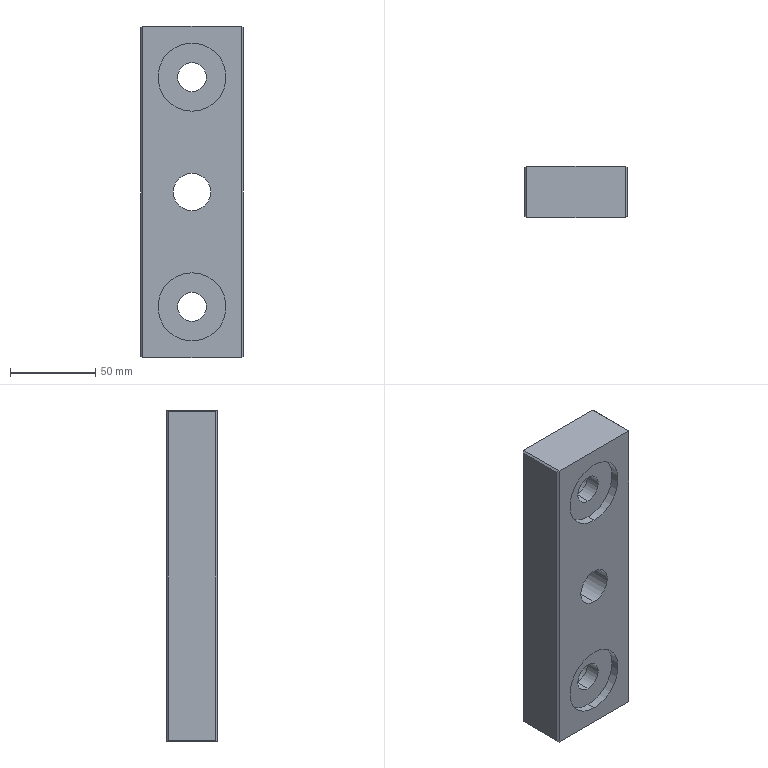Part | SolidWorks | features BaseBody 1 | 1 solid | 38 faces | box 60 x 30 x 195 mm | volume 305388 mm3 | plane 18 | cylinder 14 | cone 6 | commonest cylinder face diameters 17 x4 26 x4 40 x4 22 x2
STEP:
#1=CARTESIAN_POINT('',(0.,14.,-80.5));
#2=VERTEX_POINT('',#1);
#3=CARTESIAN_POINT('',(0.,14.,-54.5));
#4=VERTEX_POINT('',#3);
#5=CARTESIAN_POINT('',(0.,14.,-67.5));
#6=DIRECTION('',(0.,1.,0.));
#7=DIRECTION('',(0.,0.,-1.));
#8=AXIS2_PLACEMENT_3D('',#5,#6,#7);
#9=CIRCLE('',#8,13.);
#10=EDGE_CURVE('',#2,#4,#9,.T.);
#11=ORIENTED_EDGE('',*,*,#10,.F.);
#12=CARTESIAN_POINT('',(0.,15.,-81.5));
#13=VERTEX_POINT('',#12);
#14=CARTESIAN_POINT('',(0.,14.,-80.5));
#15=DIRECTION('',(0.,0.7071,-0.7071));
#16=VECTOR('',#15,1000.);
#17=LINE('',#14,#16);
#18=EDGE_CURVE('',#2,#13,#17,.T.);
#19=ORIENTED_EDGE('',*,*,#18,.T.);
#20=CARTESIAN_POINT('',(0.,15.,-53.5));
#21=VERTEX_POINT('',#20);
#22=CARTESIAN_POINT('',(0.,15.,-67.5));
#23=DIRECTION('',(0.,-1.,0.));
#24=DIRECTION('',(0.,0.,-1.));
#25=AXIS2_PLACEMENT_3D('',#22,#23,#24);
#26=CIRCLE('',#25,14.);
#27=EDGE_CURVE('',#21,#13,#26,.T.);
#28=ORIENTED_EDGE('',*,*,#27,.F.);
#29=CARTESIAN_POINT('',(0.,14.,-54.5));
#30=DIRECTION('',(0.,0.7071,0.7071));
#31=VECTOR('',#30,1000.);
#32=LINE('',#29,#31);
#33=EDGE_CURVE('',#4,#21,#32,.T.);
#34=ORIENTED_EDGE('',*,*,#33,.F.);
#35=EDGE_LOOP('',(#11,#19,#28,#34));
#36=FACE_OUTER_BOUND('',#35,.T.);
#37=CARTESIAN_POINT('',(0.,14.,-67.5));
#38=DIRECTION('',(0.,1.,0.));
#39=DIRECTION('',(0.,0.,1.));
#40=AXIS2_PLACEMENT_3D('',#37,#38,#39);
#41=CONICAL_SURFACE('',#40,13.,0.7854);
#42=ADVANCED_FACE('',(#36),#41,.F.);
#43=CARTESIAN_POINT('',(0.,14.,-11.));
#44=VERTEX_POINT('',#43);
#45=CARTESIAN_POINT('',(0.,14.,11.));
#46=VERTEX_POINT('',#45);
#47=CARTESIAN_POINT('',(0.,14.,0.));
#48=DIRECTION('',(0.,1.,0.));
#49=DIRECTION('',(0.,0.,-1.));
#50=AXIS2_PLACEMENT_3D('',#47,#48,#49);
#51=CIRCLE('',#50,11.);
#52=EDGE_CURVE('',#44,#46,#51,.T.);
#53=ORIENTED_EDGE('',*,*,#52,.F.);
#54=CARTESIAN_POINT('',(0.,15.,-12.));
#55=VERTEX_POINT('',#54);
#56=CARTESIAN_POINT('',(0.,14.,-11.));
#57=DIRECTION('',(0.,0.7071,-0.7071));
#58=VECTOR('',#57,1000.);
#59=LINE('',#56,#58);
#60=EDGE_CURVE('',#44,#55,#59,.T.);
#61=ORIENTED_EDGE('',*,*,#60,.T.);
#62=CARTESIAN_POINT('',(0.,15.,12.));
#63=VERTEX_POINT('',#62);
#64=CARTESIAN_POINT('',(0.,15.,0.));
#65=DIRECTION('',(0.,-1.,0.));
#66=DIRECTION('',(0.,0.,-1.));
#67=AXIS2_PLACEMENT_3D('',#64,#65,#66);
#68=CIRCLE('',#67,12.);
#69=EDGE_CURVE('',#63,#55,#68,.T.);
#70=ORIENTED_EDGE('',*,*,#69,.F.);
#71=CARTESIAN_POINT('',(0.,14.,11.));
#72=DIRECTION('',(0.,0.7071,0.7071));
#73=VECTOR('',#72,1000.);
#74=LINE('',#71,#73);
#75=EDGE_CURVE('',#46,#63,#74,.T.);
#76=ORIENTED_EDGE('',*,*,#75,.F.);
#77=EDGE_LOOP('',(#53,#61,#70,#76));
#78=FACE_OUTER_BOUND('',#77,.T.);
#79=CARTESIAN_POINT('',(0.,14.,0.));
#80=DIRECTION('',(0.,1.,0.));
#81=DIRECTION('',(0.,0.,1.));
#82=AXIS2_PLACEMENT_3D('',#79,#80,#81);
#83=CONICAL_SURFACE('',#82,11.,0.7854);
#84=ADVANCED_FACE('',(#78),#83,.F.);
#85=CARTESIAN_POINT('',(0.,14.,54.5));
#86=VERTEX_POINT('',#85);
#87=CARTESIAN_POINT('',(0.,14.,80.5));
#88=VERTEX_POINT('',#87);
#89=CARTESIAN_POINT('',(0.,14.,67.5));
#90=DIRECTION('',(0.,1.,0.));
#91=DIRECTION('',(0.,0.,-1.));
#92=AXIS2_PLACEMENT_3D('',#89,#90,#91);
#93=CIRCLE('',#92,13.);
#94=EDGE_CURVE('',#86,#88,#93,.T.);
#95=ORIENTED_EDGE('',*,*,#94,.F.);
#96=CARTESIAN_POINT('',(0.,15.,53.5));
#97=VERTEX_POINT('',#96);
#98=CARTESIAN_POINT('',(0.,14.,54.5));
#99=DIRECTION('',(0.,0.7071,-0.7071));
#100=VECTOR('',#99,1000.);
#101=LINE('',#98,#100);
#102=EDGE_CURVE('',#86,#97,#101,.T.);
#103=ORIENTED_EDGE('',*,*,#102,.T.);
#104=CARTESIAN_POINT('',(0.,15.,81.5));
#105=VERTEX_POINT('',#104);
#106=CARTESIAN_POINT('',(0.,15.,67.5));
#107=DIRECTION('',(0.,-1.,0.));
#108=DIRECTION('',(0.,0.,-1.));
#109=AXIS2_PLACEMENT_3D('',#106,#107,#108);
#110=CIRCLE('',#109,14.);
#111=EDGE_CURVE('',#105,#97,#110,.T.);
#112=ORIENTED_EDGE('',*,*,#111,.F.);
#113=CARTESIAN_POINT('',(0.,14.,80.5));
#114=DIRECTION('',(0.,0.7071,0.7071));
#115=VECTOR('',#114,1000.);
#116=LINE('',#113,#115);
#117=EDGE_CURVE('',#88,#105,#116,.T.);
#118=ORIENTED_EDGE('',*,*,#117,.F.);
#119=EDGE_LOOP('',(#95,#103,#112,#118));
#120=FACE_OUTER_BOUND('',#119,.T.);
#121=CARTESIAN_POINT('',(0.,14.,67.5));
#122=DIRECTION('',(0.,1.,0.));
#123=DIRECTION('',(0.,0.,1.));
#124=AXIS2_PLACEMENT_3D('',#121,#122,#123);
#125=CONICAL_SURFACE('',#124,13.,0.7854);
#126=ADVANCED_FACE('',(#120),#125,.F.);
#127=CARTESIAN_POINT('',(0.,-1.,-80.5));
#128=VERTEX_POINT('',#127);
#129=CARTESIAN_POINT('',(0.,-1.,-54.5));
#130=VERTEX_POINT('',#129);
#131=CARTESIAN_POINT('',(0.,-1.,-67.5));
#132=DIRECTION('',(0.,1.,0.));
#133=DIRECTION('',(0.,0.,1.));
#134=AXIS2_PLACEMENT_3D('',#131,#132,#133);
#135=CIRCLE('',#134,13.);
#136=EDGE_CURVE('',#128,#130,#135,.T.);
#137=ORIENTED_EDGE('',*,*,#136,.F.);
#138=CARTESIAN_POINT('',(0.,-1.,-80.5));
#139=DIRECTION('',(0.,1.,0.));
#140=VECTOR('',#139,1000.);
#141=LINE('',#138,#140);
#142=EDGE_CURVE('',#128,#2,#141,.T.);
#143=ORIENTED_EDGE('',*,*,#142,.T.);
#144=ORIENTED_EDGE('',*,*,#10,.T.);
#145=CARTESIAN_POINT('',(0.,-1.,-54.5));
#146=DIRECTION('',(0.,1.,0.));
#147=VECTOR('',#146,1000.);
#148=LINE('',#145,#147);
#149=EDGE_CURVE('',#130,#4,#148,.T.);
#150=ORIENTED_EDGE('',*,*,#149,.F.);
#151=EDGE_LOOP('',(#137,#143,#144,#150));
#152=FACE_OUTER_BOUND('',#151,.T.);
#153=CARTESIAN_POINT('',(0.,-1.,-67.5));
#154=DIRECTION('',(0.,1.,0.));
#155=DIRECTION('',(0.,0.,1.));
#156=AXIS2_PLACEMENT_3D('',#153,#154,#155);
#157=CYLINDRICAL_SURFACE('',#156,13.);
#158=ADVANCED_FACE('',(#152),#157,.F.);
#159=CARTESIAN_POINT('',(0.,-1.,54.5));
#160=VERTEX_POINT('',#159);
#161=CARTESIAN_POINT('',(0.,-1.,80.5));
#162=VERTEX_POINT('',#161);
#163=CARTESIAN_POINT('',(0.,-1.,67.5));
#164=DIRECTION('',(0.,1.,0.));
#165=DIRECTION('',(0.,0.,1.));
#166=AXIS2_PLACEMENT_3D('',#163,#164,#165);
#167=CIRCLE('',#166,13.);
#168=EDGE_CURVE('',#160,#162,#167,.T.);
#169=ORIENTED_EDGE('',*,*,#168,.F.);
#170=CARTESIAN_POINT('',(0.,-1.,54.5));
#171=DIRECTION('',(0.,1.,0.));
#172=VECTOR('',#171,1000.);
#173=LINE('',#170,#172);
#174=EDGE_CURVE('',#160,#86,#173,.T.);
#175=ORIENTED_EDGE('',*,*,#174,.T.);
#176=ORIENTED_EDGE('',*,*,#94,.T.);
#177=CARTESIAN_POINT('',(0.,-1.,80.5));
#178=DIRECTION('',(0.,1.,0.));
#179=VECTOR('',#178,1000.);
#180=LINE('',#177,#179);
#181=EDGE_CURVE('',#162,#88,#180,.T.);
#182=ORIENTED_EDGE('',*,*,#181,.F.);
#183=EDGE_LOOP('',(#169,#175,#176,#182));
#184=FACE_OUTER_BOUND('',#183,.T.);
#185=CARTESIAN_POINT('',(0.,-1.,67.5));
#186=DIRECTION('',(0.,1.,0.));
#187=DIRECTION('',(0.,0.,1.));
#188=AXIS2_PLACEMENT_3D('',#185,#186,#187);
#189=CYLINDRICAL_SURFACE('',#188,13.);
#190=ADVANCED_FACE('',(#184),#189,.F.);
#191=CARTESIAN_POINT('',(0.,-10.,87.5));
#192=VERTEX_POINT('',#191);
#193=CARTESIAN_POINT('',(0.,-10.,47.5));
#194=VERTEX_POINT('',#193);
#195=CARTESIAN_POINT('',(0.,-10.,67.5));
#196=DIRECTION('',(0.,-1.,0.));
#197=DIRECTION('',(0.,0.,-1.));
#198=AXIS2_PLACEMENT_3D('',#195,#196,#197);
#199=CIRCLE('',#198,20.);
#200=EDGE_CURVE('',#192,#194,#199,.T.);
#201=ORIENTED_EDGE('',*,*,#200,.F.);
#202=CARTESIAN_POINT('',(0.,-15.,87.5));
#203=VERTEX_POINT('',#202);
#204=CARTESIAN_POINT('',(0.,-10.,87.5));
#205=DIRECTION('',(0.,-1.,0.));
#206=VECTOR('',#205,1000.);
#207=LINE('',#204,#206);
#208=EDGE_CURVE('',#192,#203,#207,.T.);
#209=ORIENTED_EDGE('',*,*,#208,.T.);
#210=CARTESIAN_POINT('',(0.,-15.,47.5));
#211=VERTEX_POINT('',#210);
#212=CARTESIAN_POINT('',(0.,-15.,67.5));
#213=DIRECTION('',(0.,-1.,0.));
#214=DIRECTION('',(0.,0.,-1.));
#215=AXIS2_PLACEMENT_3D('',#212,#213,#214);
#216=CIRCLE('',#215,20.);
#217=EDGE_CURVE('',#203,#211,#216,.T.);
#218=ORIENTED_EDGE('',*,*,#217,.T.);
#219=CARTESIAN_POINT('',(0.,-10.,47.5));
#220=DIRECTION('',(0.,-1.,0.));
#221=VECTOR('',#220,1000.);
#222=LINE('',#219,#221);
#223=EDGE_CURVE('',#194,#211,#222,.T.);
#224=ORIENTED_EDGE('',*,*,#223,.F.);
#225=EDGE_LOOP('',(#201,#209,#218,#224));
#226=FACE_OUTER_BOUND('',#225,.T.);
#227=CARTESIAN_POINT('',(0.,-10.,67.5));
#228=DIRECTION('',(0.,-1.,0.));
#229=DIRECTION('',(0.,0.,-1.));
#230=AXIS2_PLACEMENT_3D('',#227,#228,#229);
#231=CYLINDRICAL_SURFACE('',#230,20.);
#232=ADVANCED_FACE('',(#226),#231,.F.);
#233=CARTESIAN_POINT('',(0.,-10.,-47.5));
#234=VERTEX_POINT('',#233);
#235=CARTESIAN_POINT('',(0.,-10.,-87.5));
#236=VERTEX_POINT('',#235);
#237=CARTESIAN_POINT('',(0.,-10.,-67.5));
#238=DIRECTION('',(0.,-1.,0.));
#239=DIRECTION('',(0.,0.,-1.));
#240=AXIS2_PLACEMENT_3D('',#237,#238,#239);
#241=CIRCLE('',#240,20.);
#242=EDGE_CURVE('',#234,#236,#241,.T.);
#243=ORIENTED_EDGE('',*,*,#242,.F.);
#244=CARTESIAN_POINT('',(0.,-15.,-47.5));
#245=VERTEX_POINT('',#244);
#246=CARTESIAN_POINT('',(0.,-10.,-47.5));
#247=DIRECTION('',(0.,-1.,0.));
#248=VECTOR('',#247,1000.);
#249=LINE('',#246,#248);
#250=EDGE_CURVE('',#234,#245,#249,.T.);
#251=ORIENTED_EDGE('',*,*,#250,.T.);
#252=CARTESIAN_POINT('',(0.,-15.,-87.5));
#253=VERTEX_POINT('',#252);
#254=CARTESIAN_POINT('',(0.,-15.,-67.5));
#255=DIRECTION('',(0.,-1.,0.));
#256=DIRECTION('',(0.,0.,-1.));
#257=AXIS2_PLACEMENT_3D('',#254,#255,#256);
#258=CIRCLE('',#257,20.);
#259=EDGE_CURVE('',#245,#253,#258,.T.);
#260=ORIENTED_EDGE('',*,*,#259,.T.);
#261=CARTESIAN_POINT('',(0.,-10.,-87.5));
#262=DIRECTION('',(0.,-1.,0.));
#263=VECTOR('',#262,1000.);
#264=LINE('',#261,#263);
#265=EDGE_CURVE('',#236,#253,#264,.T.);
#266=ORIENTED_EDGE('',*,*,#265,.F.);
#267=EDGE_LOOP('',(#243,#251,#260,#266));
#268=FACE_OUTER_BOUND('',#267,.T.);
#269=CARTESIAN_POINT('',(0.,-10.,-67.5));
#270=DIRECTION('',(0.,-1.,0.));
#271=DIRECTION('',(0.,0.,-1.));
#272=AXIS2_PLACEMENT_3D('',#269,#270,#271);
#273=CYLINDRICAL_SURFACE('',#272,20.);
#274=ADVANCED_FACE('',(#268),#273,.F.);
#275=ORIENTED_EDGE('',*,*,#52,.T.);
#276=CARTESIAN_POINT('',(0.,-15.,11.));
#277=VERTEX_POINT('',#276);
#278=CARTESIAN_POINT('',(0.,15.,11.));
#279=DIRECTION('',(0.,-1.,0.));
#280=VECTOR('',#279,1000.);
#281=LINE('',#278,#280);
#282=EDGE_CURVE('',#46,#277,#281,.T.);
#283=ORIENTED_EDGE('',*,*,#282,.T.);
#284=CARTESIAN_POINT('',(0.,-15.,-11.));
#285=VERTEX_POINT('',#284);
#286=CARTESIAN_POINT('',(0.,-15.,0.));
#287=DIRECTION('',(0.,1.,0.));
#288=DIRECTION('',(0.,0.,1.));
#289=AXIS2_PLACEMENT_3D('',#286,#287,#288);
#290=CIRCLE('',#289,11.);
#291=EDGE_CURVE('',#285,#277,#290,.T.);
#292=ORIENTED_EDGE('',*,*,#291,.F.);
#293=CARTESIAN_POINT('',(0.,15.,-11.));
#294=DIRECTION('',(0.,-1.,0.));
#295=VECTOR('',#294,1000.);
#296=LINE('',#293,#295);
#297=EDGE_CURVE('',#44,#285,#296,.T.);
#298=ORIENTED_EDGE('',*,*,#297,.F.);
#299=EDGE_LOOP('',(#275,#283,#292,#298));
#300=FACE_OUTER_BOUND('',#299,.T.);
#301=CARTESIAN_POINT('',(0.,15.,0.));
#302=DIRECTION('',(0.,-1.,0.));
#303=DIRECTION('',(0.,0.,-1.));
#304=AXIS2_PLACEMENT_3D('',#301,#302,#303);
#305=CYLINDRICAL_SURFACE('',#304,11.);
#306=ADVANCED_FACE('',(#300),#305,.F.);
#307=CARTESIAN_POINT('',(0.,-1.,-76.));
#308=VERTEX_POINT('',#307);
#309=CARTESIAN_POINT('',(0.,-1.,-59.));
#310=VERTEX_POINT('',#309);
#311=CARTESIAN_POINT('',(0.,-1.,-67.5));
#312=DIRECTION('',(0.,1.,0.));
#313=DIRECTION('',(0.,0.,1.));
#314=AXIS2_PLACEMENT_3D('',#311,#312,#313);
#315=CIRCLE('',#314,8.5);
#316=EDGE_CURVE('',#308,#310,#315,.T.);
#317=ORIENTED_EDGE('',*,*,#316,.T.);
#318=CARTESIAN_POINT('',(0.,-10.,-59.));
#319=VERTEX_POINT('',#318);
#320=CARTESIAN_POINT('',(0.,15.,-59.));
#321=DIRECTION('',(0.,-1.,0.));
#322=VECTOR('',#321,1000.);
#323=LINE('',#320,#322);
#324=EDGE_CURVE('',#310,#319,#323,.T.);
#325=ORIENTED_EDGE('',*,*,#324,.T.);
#326=CARTESIAN_POINT('',(0.,-10.,-76.));
#327=VERTEX_POINT('',#326);
#328=CARTESIAN_POINT('',(0.,-10.,-67.5));
#329=DIRECTION('',(0.,-1.,0.));
#330=DIRECTION('',(0.,0.,-1.));
#331=AXIS2_PLACEMENT_3D('',#328,#329,#330);
#332=CIRCLE('',#331,8.5);
#333=EDGE_CURVE('',#319,#327,#332,.T.);
#334=ORIENTED_EDGE('',*,*,#333,.T.);
#335=CARTESIAN_POINT('',(0.,15.,-76.));
#336=DIRECTION('',(0.,-1.,0.));
#337=VECTOR('',#336,1000.);
#338=LINE('',#335,#337);
#339=EDGE_CURVE('',#308,#327,#338,.T.);
#340=ORIENTED_EDGE('',*,*,#339,.F.);
#341=EDGE_LOOP('',(#317,#325,#334,#340));
#342=FACE_OUTER_BOUND('',#341,.T.);
#343=CARTESIAN_POINT('',(0.,15.,-67.5));
#344=DIRECTION('',(0.,-1.,0.));
#345=DIRECTION('',(0.,0.,-1.));
#346=AXIS2_PLACEMENT_3D('',#343,#344,#345);
#347=CYLINDRICAL_SURFACE('',#346,8.5);
#348=ADVANCED_FACE('',(#342),#347,.F.);
#349=CARTESIAN_POINT('',(0.,-1.,59.));
#350=VERTEX_POINT('',#349);
#351=CARTESIAN_POINT('',(0.,-1.,76.));
#352=VERTEX_POINT('',#351);
#353=CARTESIAN_POINT('',(0.,-1.,67.5));
#354=DIRECTION('',(0.,1.,0.));
#355=DIRECTION('',(0.,0.,1.));
#356=AXIS2_PLACEMENT_3D('',#353,#354,#355);
#357=CIRCLE('',#356,8.5);
#358=EDGE_CURVE('',#350,#352,#357,.T.);
#359=ORIENTED_EDGE('',*,*,#358,.T.);
#360=CARTESIAN_POINT('',(0.,-10.,76.));
#361=VERTEX_POINT('',#360);
#362=CARTESIAN_POINT('',(0.,15.,76.));
#363=DIRECTION('',(0.,-1.,0.));
#364=VECTOR('',#363,1000.);
#365=LINE('',#362,#364);
#366=EDGE_CURVE('',#352,#361,#365,.T.);
#367=ORIENTED_EDGE('',*,*,#366,.T.);
#368=CARTESIAN_POINT('',(0.,-10.,59.));
#369=VERTEX_POINT('',#368);
#370=CARTESIAN_POINT('',(0.,-10.,67.5));
#371=DIRECTION('',(0.,-1.,0.));
#372=DIRECTION('',(0.,0.,-1.));
#373=AXIS2_PLACEMENT_3D('',#370,#371,#372);
#374=CIRCLE('',#373,8.5);
#375=EDGE_CURVE('',#361,#369,#374,.T.);
#376=ORIENTED_EDGE('',*,*,#375,.T.);
#377=CARTESIAN_POINT('',(0.,15.,59.));
#378=DIRECTION('',(0.,-1.,0.));
#379=VECTOR('',#378,1000.);
#380=LINE('',#377,#379);
#381=EDGE_CURVE('',#350,#369,#380,.T.);
#382=ORIENTED_EDGE('',*,*,#381,.F.);
#383=EDGE_LOOP('',(#359,#367,#376,#382));
#384=FACE_OUTER_BOUND('',#383,.T.);
#385=CARTESIAN_POINT('',(0.,15.,67.5));
#386=DIRECTION('',(0.,-1.,0.));
#387=DIRECTION('',(0.,0.,-1.));
#388=AXIS2_PLACEMENT_3D('',#385,#386,#387);
#389=CYLINDRICAL_SURFACE('',#388,8.5);
#390=ADVANCED_FACE('',(#384),#389,.F.);
#391=ORIENTED_EDGE('',*,*,#366,.F.);
#392=CARTESIAN_POINT('',(0.,-1.,67.5));
#393=DIRECTION('',(0.,1.,0.));
#394=DIRECTION('',(0.,0.,1.));
#395=AXIS2_PLACEMENT_3D('',#392,#393,#394);
#396=CIRCLE('',#395,8.5);
#397=EDGE_CURVE('',#352,#350,#396,.T.);
#398=ORIENTED_EDGE('',*,*,#397,.T.);
#399=ORIENTED_EDGE('',*,*,#381,.T.);
#400=CARTESIAN_POINT('',(0.,-10.,67.5));
#401=DIRECTION('',(0.,-1.,0.));
#402=DIRECTION('',(0.,0.,-1.));
#403=AXIS2_PLACEMENT_3D('',#400,#401,#402);
#404=CIRCLE('',#403,8.5);
#405=EDGE_CURVE('',#369,#361,#404,.T.);
#406=ORIENTED_EDGE('',*,*,#405,.T.);
#407=EDGE_LOOP('',(#391,#398,#399,#406));
#408=FACE_OUTER_BOUND('',#407,.T.);
#409=CARTESIAN_POINT('',(0.,15.,67.5));
#410=DIRECTION('',(0.,-1.,0.));
#411=DIRECTION('',(0.,0.,-1.));
#412=AXIS2_PLACEMENT_3D('',#409,#410,#411);
#413=CYLINDRICAL_SURFACE('',#412,8.5);
#414=ADVANCED_FACE('',(#408),#413,.F.);
#415=ORIENTED_EDGE('',*,*,#324,.F.);
#416=CARTESIAN_POINT('',(0.,-1.,-67.5));
#417=DIRECTION('',(0.,1.,0.));
#418=DIRECTION('',(0.,0.,1.));
#419=AXIS2_PLACEMENT_3D('',#416,#417,#418);
#420=CIRCLE('',#419,8.5);
#421=EDGE_CURVE('',#310,#308,#420,.T.);
#422=ORIENTED_EDGE('',*,*,#421,.T.);
#423=ORIENTED_EDGE('',*,*,#339,.T.);
#424=CARTESIAN_POINT('',(0.,-10.,-67.5));
#425=DIRECTION('',(0.,-1.,0.));
#426=DIRECTION('',(0.,0.,-1.));
#427=AXIS2_PLACEMENT_3D('',#424,#425,#426);
#428=CIRCLE('',#427,8.5);
#429=EDGE_CURVE('',#327,#319,#428,.T.);
#430=ORIENTED_EDGE('',*,*,#429,.T.);
#431=EDGE_LOOP('',(#415,#422,#423,#430));
#432=FACE_OUTER_BOUND('',#431,.T.);
#433=CARTESIAN_POINT('',(0.,15.,-67.5));
#434=DIRECTION('',(0.,-1.,0.));
#435=DIRECTION('',(0.,0.,-1.));
#436=AXIS2_PLACEMENT_3D('',#433,#434,#435);
#437=CYLINDRICAL_SURFACE('',#436,8.5);
#438=ADVANCED_FACE('',(#432),#437,.F.);
#439=ORIENTED_EDGE('',*,*,#111,.T.);
#440=CARTESIAN_POINT('',(0.,15.,67.5));
#441=DIRECTION('',(0.,-1.,0.));
#442=DIRECTION('',(0.,0.,-1.));
#443=AXIS2_PLACEMENT_3D('',#440,#441,#442);
#444=CIRCLE('',#443,14.);
#445=EDGE_CURVE('',#97,#105,#444,.T.);
#446=ORIENTED_EDGE('',*,*,#445,.T.);
#447=EDGE_LOOP('',(#439,#446));
#448=FACE_BOUND('',#447,.T.);
#449=ORIENTED_EDGE('',*,*,#69,.T.);
#450=CARTESIAN_POINT('',(0.,15.,0.));
#451=DIRECTION('',(0.,-1.,0.));
#452=DIRECTION('',(0.,0.,-1.));
#453=AXIS2_PLACEMENT_3D('',#450,#451,#452);
#454=CIRCLE('',#453,12.);
#455=EDGE_CURVE('',#55,#63,#454,.T.);
#456=ORIENTED_EDGE('',*,*,#455,.T.);
#457=EDGE_LOOP('',(#449,#456));
#458=FACE_BOUND('',#457,.T.);
#459=ORIENTED_EDGE('',*,*,#27,.T.);
#460=CARTESIAN_POINT('',(0.,15.,-67.5));
#461=DIRECTION('',(0.,-1.,0.));
#462=DIRECTION('',(0.,0.,-1.));
#463=AXIS2_PLACEMENT_3D('',#460,#461,#462);
#464=CIRCLE('',#463,14.);
#465=EDGE_CURVE('',#13,#21,#464,.T.);
#466=ORIENTED_EDGE('',*,*,#465,.T.);
#467=EDGE_LOOP('',(#459,#466));
#468=FACE_BOUND('',#467,.T.);
#469=CARTESIAN_POINT('',(-29.,15.,97.5));
#470=VERTEX_POINT('',#469);
#471=CARTESIAN_POINT('',(29.,15.,97.5));
#472=VERTEX_POINT('',#471);
#473=CARTESIAN_POINT('',(29.,15.,97.5));
#474=DIRECTION('',(1.,0.,0.));
#475=VECTOR('',#474,1000.);
#476=LINE('',#473,#475);
#477=EDGE_CURVE('',#470,#472,#476,.T.);
#478=ORIENTED_EDGE('',*,*,#477,.T.);
#479=CARTESIAN_POINT('',(29.,15.,-97.5));
#480=VERTEX_POINT('',#479);
#481=CARTESIAN_POINT('',(29.,15.,0.));
#482=DIRECTION('',(0.,0.,-1.));
#483=VECTOR('',#482,1000.);
#484=LINE('',#481,#483);
#485=EDGE_CURVE('',#472,#480,#484,.T.);
#486=ORIENTED_EDGE('',*,*,#485,.T.);
#487=CARTESIAN_POINT('',(-29.,15.,-97.5));
#488=VERTEX_POINT('',#487);
#489=CARTESIAN_POINT('',(-29.,15.,-97.5));
#490=DIRECTION('',(-1.,0.,0.));
#491=VECTOR('',#490,1000.);
#492=LINE('',#489,#491);
#493=EDGE_CURVE('',#480,#488,#492,.T.);
#494=ORIENTED_EDGE('',*,*,#493,.T.);
#495=CARTESIAN_POINT('',(-29.,15.,0.));
#496=DIRECTION('',(0.,0.,1.));
#497=VECTOR('',#496,1000.);
#498=LINE('',#495,#497);
#499=EDGE_CURVE('',#488,#470,#498,.T.);
#500=ORIENTED_EDGE('',*,*,#499,.T.);
#501=EDGE_LOOP('',(#478,#486,#494,#500));
#502=FACE_OUTER_BOUND('',#501,.T.);
#503=CARTESIAN_POINT('',(0.,15.,0.));
#504=DIRECTION('',(0.,-1.,0.));
#505=DIRECTION('',(0.,0.,-1.));
#506=AXIS2_PLACEMENT_3D('',#503,#504,#505);
#507=PLANE('',#506);
#508=ADVANCED_FACE('',(#448,#458,#468,#502),#507,.F.);
#509=CARTESIAN_POINT('',(0.,-15.,-67.5));
#510=DIRECTION('',(0.,-1.,0.));
#511=DIRECTION('',(0.,0.,-1.));
#512=AXIS2_PLACEMENT_3D('',#509,#510,#511);
#513=CIRCLE('',#512,20.);
#514=EDGE_CURVE('',#253,#245,#513,.T.);
#515=ORIENTED_EDGE('',*,*,#514,.F.);
#516=ORIENTED_EDGE('',*,*,#259,.F.);
#517=EDGE_LOOP('',(#515,#516));
#518=FACE_BOUND('',#517,.T.);
#519=CARTESIAN_POINT('',(0.,-15.,67.5));
#520=DIRECTION('',(0.,-1.,0.));
#521=DIRECTION('',(0.,0.,-1.));
#522=AXIS2_PLACEMENT_3D('',#519,#520,#521);
#523=CIRCLE('',#522,20.);
#524=EDGE_CURVE('',#211,#203,#523,.T.);
#525=ORIENTED_EDGE('',*,*,#524,.F.);
#526=ORIENTED_EDGE('',*,*,#217,.F.);
#527=EDGE_LOOP('',(#525,#526));
#528=FACE_BOUND('',#527,.T.);
#529=CARTESIAN_POINT('',(-29.,-15.,97.5));
#530=VERTEX_POINT('',#529);
#531=CARTESIAN_POINT('',(29.,-15.,97.5));
#532=VERTEX_POINT('',#531);
#533=CARTESIAN_POINT('',(29.,-15.,97.5));
#534=DIRECTION('',(1.,0.,0.));
#535=VECTOR('',#534,1000.);
#536=LINE('',#533,#535);
#537=EDGE_CURVE('',#530,#532,#536,.T.);
#538=ORIENTED_EDGE('',*,*,#537,.F.);
#539=CARTESIAN_POINT('',(-29.,-15.,-97.5));
#540=VERTEX_POINT('',#539);
#541=CARTESIAN_POINT('',(-29.,-15.,-96.5));
#542=DIRECTION('',(0.,0.,-1.));
#543=VECTOR('',#542,1000.);
#544=LINE('',#541,#543);
#545=EDGE_CURVE('',#530,#540,#544,.T.);
#546=ORIENTED_EDGE('',*,*,#545,.T.);
#547=CARTESIAN_POINT('',(29.,-15.,-97.5));
#548=VERTEX_POINT('',#547);
#549=CARTESIAN_POINT('',(-29.,-15.,-97.5));
#550=DIRECTION('',(-1.,0.,0.));
#551=VECTOR('',#550,1000.);
#552=LINE('',#549,#551);
#553=EDGE_CURVE('',#548,#540,#552,.T.);
#554=ORIENTED_EDGE('',*,*,#553,.F.);
#555=CARTESIAN_POINT('',(29.,-15.,96.5));
#556=DIRECTION('',(0.,0.,1.));
#557=VECTOR('',#556,1000.);
#558=LINE('',#555,#557);
#559=EDGE_CURVE('',#548,#532,#558,.T.);
#560=ORIENTED_EDGE('',*,*,#559,.T.);
#561=EDGE_LOOP('',(#538,#546,#554,#560));
#562=FACE_OUTER_BOUND('',#561,.T.);
#563=ORIENTED_EDGE('',*,*,#291,.T.);
#564=CARTESIAN_POINT('',(0.,-15.,0.));
#565=DIRECTION('',(0.,1.,0.));
#566=DIRECTION('',(0.,0.,1.));
#567=AXIS2_PLACEMENT_3D('',#564,#565,#566);
#568=CIRCLE('',#567,11.);
#569=EDGE_CURVE('',#277,#285,#568,.T.);
#570=ORIENTED_EDGE('',*,*,#569,.T.);
#571=EDGE_LOOP('',(#563,#570));
#572=FACE_BOUND('',#571,.T.);
#573=CARTESIAN_POINT('',(0.,-15.,0.));
#574=DIRECTION('',(0.,-1.,0.));
#575=DIRECTION('',(0.,0.,-1.));
#576=AXIS2_PLACEMENT_3D('',#573,#574,#575);
#577=PLANE('',#576);
#578=ADVANCED_FACE('',(#518,#528,#562,#572),#577,.T.);
#579=CARTESIAN_POINT('',(-29.,15.,-97.5));
#580=DIRECTION('',(0.,-1.,0.));
#581=VECTOR('',#580,1000.);
#582=LINE('',#579,#581);
#583=EDGE_CURVE('',#488,#540,#582,.T.);
#584=ORIENTED_EDGE('',*,*,#583,.T.);
#585=CARTESIAN_POINT('',(-30.,-14.,-96.5));
#586=VERTEX_POINT('',#585);
#587=CARTESIAN_POINT('',(-94.333,50.333,-32.167));
#588=DIRECTION('',(-0.5774,0.5774,0.5774));
#589=VECTOR('',#588,1000.);
#590=LINE('',#587,#589);
#591=EDGE_CURVE('',#540,#586,#590,.T.);
#592=ORIENTED_EDGE('',*,*,#591,.T.);
#593=CARTESIAN_POINT('',(-30.,14.,-96.5));
#594=VERTEX_POINT('',#593);
#595=CARTESIAN_POINT('',(-30.,15.,-96.5));
#596=DIRECTION('',(0.,-1.,0.));
#597=VECTOR('',#596,1000.);
#598=LINE('',#595,#597);
#599=EDGE_CURVE('',#594,#586,#598,.T.);
#600=ORIENTED_EDGE('',*,*,#599,.F.);
#601=CARTESIAN_POINT('',(-61.5,-17.5,-65.));
#602=DIRECTION('',(0.5774,0.5774,-0.5774));
#603=VECTOR('',#602,1000.);
#604=LINE('',#601,#603);
#605=EDGE_CURVE('',#594,#488,#604,.T.);
#606=ORIENTED_EDGE('',*,*,#605,.T.);
#607=EDGE_LOOP('',(#584,#592,#600,#606));
#608=FACE_OUTER_BOUND('',#607,.T.);
#609=CARTESIAN_POINT('',(-30.,15.,-96.5));
#610=DIRECTION('',(0.7071,0.,0.7071));
#611=DIRECTION('',(0.7071,0.,-0.7071));
#612=AXIS2_PLACEMENT_3D('',#609,#610,#611);
#613=PLANE('',#612);
#614=ADVANCED_FACE('',(#608),#613,.F.);
#615=ORIENTED_EDGE('',*,*,#599,.T.);
#616=CARTESIAN_POINT('',(-30.,-14.,96.5));
#617=VERTEX_POINT('',#616);
#618=CARTESIAN_POINT('',(-30.,-14.,96.5));
#619=DIRECTION('',(0.,0.,1.));
#620=VECTOR('',#619,1000.);
#621=LINE('',#618,#620);
#622=EDGE_CURVE('',#586,#617,#621,.T.);
#623=ORIENTED_EDGE('',*,*,#622,.T.);
#624=CARTESIAN_POINT('',(-30.,14.,96.5));
#625=VERTEX_POINT('',#624);
#626=CARTESIAN_POINT('',(-30.,15.,96.5));
#627=DIRECTION('',(0.,-1.,0.));
#628=VECTOR('',#627,1000.);
#629=LINE('',#626,#628);
#630=EDGE_CURVE('',#625,#617,#629,.T.);
#631=ORIENTED_EDGE('',*,*,#630,.F.);
#632=CARTESIAN_POINT('',(-30.,14.,96.5));
#633=DIRECTION('',(0.,0.,-1.));
#634=VECTOR('',#633,1000.);
#635=LINE('',#632,#634);
#636=EDGE_CURVE('',#625,#594,#635,.T.);
#637=ORIENTED_EDGE('',*,*,#636,.T.);
#638=EDGE_LOOP('',(#615,#623,#631,#637));
#639=FACE_OUTER_BOUND('',#638,.T.);
#640=CARTESIAN_POINT('',(-30.,15.,96.5));
#641=DIRECTION('',(1.,0.,0.));
#642=DIRECTION('',(0.,0.,-1.));
#643=AXIS2_PLACEMENT_3D('',#640,#641,#642);
#644=PLANE('',#643);
#645=ADVANCED_FACE('',(#639),#644,.F.);
#646=ORIENTED_EDGE('',*,*,#630,.T.);
#647=CARTESIAN_POINT('',(-30.,-14.,96.5));
#648=DIRECTION('',(0.5774,-0.5774,0.5774));
#649=VECTOR('',#648,1000.);
#650=LINE('',#647,#649);
#651=EDGE_CURVE('',#617,#530,#650,.T.);
#652=ORIENTED_EDGE('',*,*,#651,.T.);
#653=CARTESIAN_POINT('',(-29.,15.,97.5));
#654=DIRECTION('',(0.,-1.,0.));
#655=VECTOR('',#654,1000.);
#656=LINE('',#653,#655);
#657=EDGE_CURVE('',#470,#530,#656,.T.);
#658=ORIENTED_EDGE('',*,*,#657,.F.);
#659=CARTESIAN_POINT('',(-61.5,-17.5,65.));
#660=DIRECTION('',(-0.5774,-0.5774,-0.5774));
#661=VECTOR('',#660,1000.);
#662=LINE('',#659,#661);
#663=EDGE_CURVE('',#470,#625,#662,.T.);
#664=ORIENTED_EDGE('',*,*,#663,.T.);
#665=EDGE_LOOP('',(#646,#652,#658,#664));
#666=FACE_OUTER_BOUND('',#665,.T.);
#667=CARTESIAN_POINT('',(-29.,15.,97.5));
#668=DIRECTION('',(0.7071,0.,-0.7071));
#669=DIRECTION('',(-0.7071,0.,-0.7071));
#670=AXIS2_PLACEMENT_3D('',#667,#668,#669);
#671=PLANE('',#670);
#672=ADVANCED_FACE('',(#666),#671,.F.);
#673=ORIENTED_EDGE('',*,*,#537,.T.);
#674=CARTESIAN_POINT('',(29.,15.,97.5));
#675=DIRECTION('',(0.,-1.,0.));
#676=VECTOR('',#675,1000.);
#677=LINE('',#674,#676);
#678=EDGE_CURVE('',#472,#532,#677,.T.);
#679=ORIENTED_EDGE('',*,*,#678,.F.);
#680=ORIENTED_EDGE('',*,*,#477,.F.);
#681=ORIENTED_EDGE('',*,*,#657,.T.);
#682=EDGE_LOOP('',(#673,#679,#680,#681));
#683=FACE_OUTER_BOUND('',#682,.T.);
#684=CARTESIAN_POINT('',(29.,15.,97.5));
#685=DIRECTION('',(0.,0.,-1.));
#686=DIRECTION('',(-1.,0.,0.));
#687=AXIS2_PLACEMENT_3D('',#684,#685,#686);
#688=PLANE('',#687);
#689=ADVANCED_FACE('',(#683),#688,.F.);
#690=ORIENTED_EDGE('',*,*,#678,.T.);
#691=CARTESIAN_POINT('',(30.,-14.,96.5));
#692=VERTEX_POINT('',#691);
#693=CARTESIAN_POINT('',(94.333,50.333,32.167));
#694=DIRECTION('',(0.5774,0.5774,-0.5774));
#695=VECTOR('',#694,1000.);
#696=LINE('',#693,#695);
#697=EDGE_CURVE('',#532,#692,#696,.T.);
#698=ORIENTED_EDGE('',*,*,#697,.T.);
#699=CARTESIAN_POINT('',(30.,14.,96.5));
#700=VERTEX_POINT('',#699);
#701=CARTESIAN_POINT('',(30.,15.,96.5));
#702=DIRECTION('',(0.,-1.,0.));
#703=VECTOR('',#702,1000.);
#704=LINE('',#701,#703);
#705=EDGE_CURVE('',#700,#692,#704,.T.);
#706=ORIENTED_EDGE('',*,*,#705,.F.);
#707=CARTESIAN_POINT('',(61.5,-17.5,65.));
#708=DIRECTION('',(-0.5774,0.5774,0.5774));
#709=VECTOR('',#708,1000.);
#710=LINE('',#707,#709);
#711=EDGE_CURVE('',#700,#472,#710,.T.);
#712=ORIENTED_EDGE('',*,*,#711,.T.);
#713=EDGE_LOOP('',(#690,#698,#706,#712));
#714=FACE_OUTER_BOUND('',#713,.T.);
#715=CARTESIAN_POINT('',(30.,15.,96.5));
#716=DIRECTION('',(-0.7071,0.,-0.7071));
#717=DIRECTION('',(-0.7071,0.,0.7071));
#718=AXIS2_PLACEMENT_3D('',#715,#716,#717);
#719=PLANE('',#718);
#720=ADVANCED_FACE('',(#714),#719,.F.);
#721=ORIENTED_EDGE('',*,*,#705,.T.);
#722=CARTESIAN_POINT('',(30.,-14.,-96.5));
#723=VERTEX_POINT('',#722);
#724=CARTESIAN_POINT('',(30.,-14.,-96.5));
#725=DIRECTION('',(0.,0.,-1.));
#726=VECTOR('',#725,1000.);
#727=LINE('',#724,#726);
#728=EDGE_CURVE('',#692,#723,#727,.T.);
#729=ORIENTED_EDGE('',*,*,#728,.T.);
#730=CARTESIAN_POINT('',(30.,14.,-96.5));
#731=VERTEX_POINT('',#730);
#732=CARTESIAN_POINT('',(30.,15.,-96.5));
#733=DIRECTION('',(0.,-1.,0.));
#734=VECTOR('',#733,1000.);
#735=LINE('',#732,#734);
#736=EDGE_CURVE('',#731,#723,#735,.T.);
#737=ORIENTED_EDGE('',*,*,#736,.F.);
#738=CARTESIAN_POINT('',(30.,14.,-96.5));
#739=DIRECTION('',(0.,0.,1.));
#740=VECTOR('',#739,1000.);
#741=LINE('',#738,#740);
#742=EDGE_CURVE('',#731,#700,#741,.T.);
#743=ORIENTED_EDGE('',*,*,#742,.T.);
#744=EDGE_LOOP('',(#721,#729,#737,#743));
#745=FACE_OUTER_BOUND('',#744,.T.);
#746=CARTESIAN_POINT('',(30.,15.,-96.5));
#747=DIRECTION('',(-1.,0.,0.));
#748=DIRECTION('',(0.,0.,1.));
#749=AXIS2_PLACEMENT_3D('',#746,#747,#748);
#750=PLANE('',#749);
#751=ADVANCED_FACE('',(#745),#750,.F.);
#752=ORIENTED_EDGE('',*,*,#736,.T.);
#753=CARTESIAN_POINT('',(30.,-14.,-96.5));
#754=DIRECTION('',(-0.5774,-0.5774,-0.5774));
#755=VECTOR('',#754,1000.);
#756=LINE('',#753,#755);
#757=EDGE_CURVE('',#723,#548,#756,.T.);
#758=ORIENTED_EDGE('',*,*,#757,.T.);
#759=CARTESIAN_POINT('',(29.,15.,-97.5));
#760=DIRECTION('',(0.,-1.,0.));
#761=VECTOR('',#760,1000.);
#762=LINE('',#759,#761);
#763=EDGE_CURVE('',#480,#548,#762,.T.);
#764=ORIENTED_EDGE('',*,*,#763,.F.);
#765=CARTESIAN_POINT('',(61.5,-17.5,-65.));
#766=DIRECTION('',(0.5774,-0.5774,0.5774));
#767=VECTOR('',#766,1000.);
#768=LINE('',#765,#767);
#769=EDGE_CURVE('',#480,#731,#768,.T.);
#770=ORIENTED_EDGE('',*,*,#769,.T.);
#771=EDGE_LOOP('',(#752,#758,#764,#770));
#772=FACE_OUTER_BOUND('',#771,.T.);
#773=CARTESIAN_POINT('',(29.,15.,-97.5));
#774=DIRECTION('',(-0.7071,0.,0.7071));
#775=DIRECTION('',(0.7071,0.,0.7071));
#776=AXIS2_PLACEMENT_3D('',#773,#774,#775);
#777=PLANE('',#776);
#778=ADVANCED_FACE('',(#772),#777,.F.);
#779=ORIENTED_EDGE('',*,*,#553,.T.);
#780=ORIENTED_EDGE('',*,*,#583,.F.);
#781=ORIENTED_EDGE('',*,*,#493,.F.);
#782=ORIENTED_EDGE('',*,*,#763,.T.);
#783=EDGE_LOOP('',(#779,#780,#781,#782));
#784=FACE_OUTER_BOUND('',#783,.T.);
#785=CARTESIAN_POINT('',(-29.,15.,-97.5));
#786=DIRECTION('',(0.,0.,1.));
#787=DIRECTION('',(1.,0.,0.));
#788=AXIS2_PLACEMENT_3D('',#785,#786,#787);
#789=PLANE('',#788);
#790=ADVANCED_FACE('',(#784),#789,.F.);
#791=ORIENTED_EDGE('',*,*,#282,.F.);
#792=CARTESIAN_POINT('',(0.,14.,0.));
#793=DIRECTION('',(0.,1.,0.));
#794=DIRECTION('',(0.,0.,-1.));
#795=AXIS2_PLACEMENT_3D('',#792,#793,#794);
#796=CIRCLE('',#795,11.);
#797=EDGE_CURVE('',#46,#44,#796,.T.);
#798=ORIENTED_EDGE('',*,*,#797,.T.);
#799=ORIENTED_EDGE('',*,*,#297,.T.);
#800=ORIENTED_EDGE('',*,*,#569,.F.);
#801=EDGE_LOOP('',(#791,#798,#799,#800));
#802=FACE_OUTER_BOUND('',#801,.T.);
#803=CARTESIAN_POINT('',(0.,15.,0.));
#804=DIRECTION('',(0.,-1.,0.));
#805=DIRECTION('',(0.,0.,-1.));
#806=AXIS2_PLACEMENT_3D('',#803,#804,#805);
#807=CYLINDRICAL_SURFACE('',#806,11.);
#808=ADVANCED_FACE('',(#802),#807,.F.);
#809=ORIENTED_EDGE('',*,*,#250,.F.);
#810=CARTESIAN_POINT('',(0.,-10.,-67.5));
#811=DIRECTION('',(0.,-1.,0.));
#812=DIRECTION('',(0.,0.,-1.));
#813=AXIS2_PLACEMENT_3D('',#810,#811,#812);
#814=CIRCLE('',#813,20.);
#815=EDGE_CURVE('',#236,#234,#814,.T.);
#816=ORIENTED_EDGE('',*,*,#815,.F.);
#817=ORIENTED_EDGE('',*,*,#265,.T.);
#818=ORIENTED_EDGE('',*,*,#514,.T.);
#819=EDGE_LOOP('',(#809,#816,#817,#818));
#820=FACE_OUTER_BOUND('',#819,.T.);
#821=CARTESIAN_POINT('',(0.,-10.,-67.5));
#822=DIRECTION('',(0.,-1.,0.));
#823=DIRECTION('',(0.,0.,-1.));
#824=AXIS2_PLACEMENT_3D('',#821,#822,#823);
#825=CYLINDRICAL_SURFACE('',#824,20.);
#826=ADVANCED_FACE('',(#820),#825,.F.);
#827=ORIENTED_EDGE('',*,*,#429,.F.);
#828=ORIENTED_EDGE('',*,*,#333,.F.);
#829=EDGE_LOOP('',(#827,#828));
#830=FACE_BOUND('',#829,.T.);
#831=ORIENTED_EDGE('',*,*,#815,.T.);
#832=ORIENTED_EDGE('',*,*,#242,.T.);
#833=EDGE_LOOP('',(#831,#832));
#834=FACE_OUTER_BOUND('',#833,.T.);
#835=CARTESIAN_POINT('',(0.,-10.,-67.5));
#836=DIRECTION('',(0.,-1.,0.));
#837=DIRECTION('',(0.,0.,-1.));
#838=AXIS2_PLACEMENT_3D('',#835,#836,#837);
#839=PLANE('',#838);
#840=ADVANCED_FACE('',(#830,#834),#839,.T.);
#841=ORIENTED_EDGE('',*,*,#208,.F.);
#842=CARTESIAN_POINT('',(0.,-10.,67.5));
#843=DIRECTION('',(0.,-1.,0.));
#844=DIRECTION('',(0.,0.,-1.));
#845=AXIS2_PLACEMENT_3D('',#842,#843,#844);
#846=CIRCLE('',#845,20.);
#847=EDGE_CURVE('',#194,#192,#846,.T.);
#848=ORIENTED_EDGE('',*,*,#847,.F.);
#849=ORIENTED_EDGE('',*,*,#223,.T.);
#850=ORIENTED_EDGE('',*,*,#524,.T.);
#851=EDGE_LOOP('',(#841,#848,#849,#850));
#852=FACE_OUTER_BOUND('',#851,.T.);
#853=CARTESIAN_POINT('',(0.,-10.,67.5));
#854=DIRECTION('',(0.,-1.,0.));
#855=DIRECTION('',(0.,0.,-1.));
#856=AXIS2_PLACEMENT_3D('',#853,#854,#855);
#857=CYLINDRICAL_SURFACE('',#856,20.);
#858=ADVANCED_FACE('',(#852),#857,.F.);
#859=ORIENTED_EDGE('',*,*,#405,.F.);
#860=ORIENTED_EDGE('',*,*,#375,.F.);
#861=EDGE_LOOP('',(#859,#860));
#862=FACE_BOUND('',#861,.T.);
#863=ORIENTED_EDGE('',*,*,#847,.T.);
#864=ORIENTED_EDGE('',*,*,#200,.T.);
#865=EDGE_LOOP('',(#863,#864));
#866=FACE_OUTER_BOUND('',#865,.T.);
#867=CARTESIAN_POINT('',(0.,-10.,67.5));
#868=DIRECTION('',(0.,-1.,0.));
#869=DIRECTION('',(0.,0.,-1.));
#870=AXIS2_PLACEMENT_3D('',#867,#868,#869);
#871=PLANE('',#870);
#872=ADVANCED_FACE('',(#862,#866),#871,.T.);
#873=ORIENTED_EDGE('',*,*,#174,.F.);
#874=CARTESIAN_POINT('',(0.,-1.,67.5));
#875=DIRECTION('',(0.,1.,0.));
#876=DIRECTION('',(0.,0.,1.));
#877=AXIS2_PLACEMENT_3D('',#874,#875,#876);
#878=CIRCLE('',#877,13.);
#879=EDGE_CURVE('',#162,#160,#878,.T.);
#880=ORIENTED_EDGE('',*,*,#879,.F.);
#881=ORIENTED_EDGE('',*,*,#181,.T.);
#882=CARTESIAN_POINT('',(0.,14.,67.5));
#883=DIRECTION('',(0.,1.,0.));
#884=DIRECTION('',(0.,0.,-1.));
#885=AXIS2_PLACEMENT_3D('',#882,#883,#884);
#886=CIRCLE('',#885,13.);
#887=EDGE_CURVE('',#88,#86,#886,.T.);
#888=ORIENTED_EDGE('',*,*,#887,.T.);
#889=EDGE_LOOP('',(#873,#880,#881,#888));
#890=FACE_OUTER_BOUND('',#889,.T.);
#891=CARTESIAN_POINT('',(0.,-1.,67.5));
#892=DIRECTION('',(0.,1.,0.));
#893=DIRECTION('',(0.,0.,1.));
#894=AXIS2_PLACEMENT_3D('',#891,#892,#893);
#895=CYLINDRICAL_SURFACE('',#894,13.);
#896=ADVANCED_FACE('',(#890),#895,.F.);
#897=ORIENTED_EDGE('',*,*,#358,.F.);
#898=ORIENTED_EDGE('',*,*,#397,.F.);
#899=EDGE_LOOP('',(#897,#898));
#900=FACE_BOUND('',#899,.T.);
#901=ORIENTED_EDGE('',*,*,#879,.T.);
#902=ORIENTED_EDGE('',*,*,#168,.T.);
#903=EDGE_LOOP('',(#901,#902));
#904=FACE_OUTER_BOUND('',#903,.T.);
#905=CARTESIAN_POINT('',(0.,-1.,67.5));
#906=DIRECTION('',(0.,1.,0.));
#907=DIRECTION('',(0.,0.,1.));
#908=AXIS2_PLACEMENT_3D('',#905,#906,#907);
#909=PLANE('',#908);
#910=ADVANCED_FACE('',(#900,#904),#909,.T.);
#911=ORIENTED_EDGE('',*,*,#142,.F.);
#912=CARTESIAN_POINT('',(0.,-1.,-67.5));
#913=DIRECTION('',(0.,1.,0.));
#914=DIRECTION('',(0.,0.,1.));
#915=AXIS2_PLACEMENT_3D('',#912,#913,#914);
#916=CIRCLE('',#915,13.);
#917=EDGE_CURVE('',#130,#128,#916,.T.);
#918=ORIENTED_EDGE('',*,*,#917,.F.);
#919=ORIENTED_EDGE('',*,*,#149,.T.);
#920=CARTESIAN_POINT('',(0.,14.,-67.5));
#921=DIRECTION('',(0.,1.,0.));
#922=DIRECTION('',(0.,0.,-1.));
#923=AXIS2_PLACEMENT_3D('',#920,#921,#922);
#924=CIRCLE('',#923,13.);
#925=EDGE_CURVE('',#4,#2,#924,.T.);
#926=ORIENTED_EDGE('',*,*,#925,.T.);
#927=EDGE_LOOP('',(#911,#918,#919,#926));
#928=FACE_OUTER_BOUND('',#927,.T.);
#929=CARTESIAN_POINT('',(0.,-1.,-67.5));
#930=DIRECTION('',(0.,1.,0.));
#931=DIRECTION('',(0.,0.,1.));
#932=AXIS2_PLACEMENT_3D('',#929,#930,#931);
#933=CYLINDRICAL_SURFACE('',#932,13.);
#934=ADVANCED_FACE('',(#928),#933,.F.);
#935=ORIENTED_EDGE('',*,*,#316,.F.);
#936=ORIENTED_EDGE('',*,*,#421,.F.);
#937=EDGE_LOOP('',(#935,#936));
#938=FACE_BOUND('',#937,.T.);
#939=ORIENTED_EDGE('',*,*,#917,.T.);
#940=ORIENTED_EDGE('',*,*,#136,.T.);
#941=EDGE_LOOP('',(#939,#940));
#942=FACE_OUTER_BOUND('',#941,.T.);
#943=CARTESIAN_POINT('',(0.,-1.,-67.5));
#944=DIRECTION('',(0.,1.,0.));
#945=DIRECTION('',(0.,0.,1.));
#946=AXIS2_PLACEMENT_3D('',#943,#944,#945);
#947=PLANE('',#946);
#948=ADVANCED_FACE('',(#938,#942),#947,.T.);
#949=ORIENTED_EDGE('',*,*,#102,.F.);
#950=ORIENTED_EDGE('',*,*,#887,.F.);
#951=ORIENTED_EDGE('',*,*,#117,.T.);
#952=ORIENTED_EDGE('',*,*,#445,.F.);
#953=EDGE_LOOP('',(#949,#950,#951,#952));
#954=FACE_OUTER_BOUND('',#953,.T.);
#955=CARTESIAN_POINT('',(0.,14.,67.5));
#956=DIRECTION('',(0.,1.,0.));
#957=DIRECTION('',(0.,0.,1.));
#958=AXIS2_PLACEMENT_3D('',#955,#956,#957);
#959=CONICAL_SURFACE('',#958,13.,0.7854);
#960=ADVANCED_FACE('',(#954),#959,.F.);
#961=ORIENTED_EDGE('',*,*,#60,.F.);
#962=ORIENTED_EDGE('',*,*,#797,.F.);
#963=ORIENTED_EDGE('',*,*,#75,.T.);
#964=ORIENTED_EDGE('',*,*,#455,.F.);
#965=EDGE_LOOP('',(#961,#962,#963,#964));
#966=FACE_OUTER_BOUND('',#965,.T.);
#967=CARTESIAN_POINT('',(0.,14.,0.));
#968=DIRECTION('',(0.,1.,0.));
#969=DIRECTION('',(0.,0.,1.));
#970=AXIS2_PLACEMENT_3D('',#967,#968,#969);
#971=CONICAL_SURFACE('',#970,11.,0.7854);
#972=ADVANCED_FACE('',(#966),#971,.F.);
#973=ORIENTED_EDGE('',*,*,#18,.F.);
#974=ORIENTED_EDGE('',*,*,#925,.F.);
#975=ORIENTED_EDGE('',*,*,#33,.T.);
#976=ORIENTED_EDGE('',*,*,#465,.F.);
#977=EDGE_LOOP('',(#973,#974,#975,#976));
#978=FACE_OUTER_BOUND('',#977,.T.);
#979=CARTESIAN_POINT('',(0.,14.,-67.5));
#980=DIRECTION('',(0.,1.,0.));
#981=DIRECTION('',(0.,0.,1.));
#982=AXIS2_PLACEMENT_3D('',#979,#980,#981);
#983=CONICAL_SURFACE('',#982,13.,0.7854);
#984=ADVANCED_FACE('',(#978),#983,.F.);
#985=ORIENTED_EDGE('',*,*,#591,.F.);
#986=ORIENTED_EDGE('',*,*,#545,.F.);
#987=ORIENTED_EDGE('',*,*,#651,.F.);
#988=ORIENTED_EDGE('',*,*,#622,.F.);
#989=EDGE_LOOP('',(#985,#986,#987,#988));
#990=FACE_OUTER_BOUND('',#989,.T.);
#991=CARTESIAN_POINT('',(-30.,-14.,96.5));
#992=DIRECTION('',(-0.7071,-0.7071,0.));
#993=DIRECTION('',(0.,0.,-1.));
#994=AXIS2_PLACEMENT_3D('',#991,#992,#993);
#995=PLANE('',#994);
#996=ADVANCED_FACE('',(#990),#995,.T.);
#997=ORIENTED_EDGE('',*,*,#697,.F.);
#998=ORIENTED_EDGE('',*,*,#559,.F.);
#999=ORIENTED_EDGE('',*,*,#757,.F.);
#1000=ORIENTED_EDGE('',*,*,#728,.F.);
#1001=EDGE_LOOP('',(#997,#998,#999,#1000));
#1002=FACE_OUTER_BOUND('',#1001,.T.);
#1003=CARTESIAN_POINT('',(30.,-14.,-96.5));
#1004=DIRECTION('',(0.7071,-0.7071,0.));
#1005=DIRECTION('',(0.,0.,1.));
#1006=AXIS2_PLACEMENT_3D('',#1003,#1004,#1005);
#1007=PLANE('',#1006);
#1008=ADVANCED_FACE('',(#1002),#1007,.T.);
#1009=ORIENTED_EDGE('',*,*,#711,.F.);
#1010=ORIENTED_EDGE('',*,*,#742,.F.);
#1011=ORIENTED_EDGE('',*,*,#769,.F.);
#1012=ORIENTED_EDGE('',*,*,#485,.F.);
#1013=EDGE_LOOP('',(#1009,#1010,#1011,#1012));
#1014=FACE_OUTER_BOUND('',#1013,.T.);
#1015=CARTESIAN_POINT('',(29.,15.,0.));
#1016=DIRECTION('',(-0.7071,-0.7071,0.));
#1017=DIRECTION('',(0.,0.,-1.));
#1018=AXIS2_PLACEMENT_3D('',#1015,#1016,#1017);
#1019=PLANE('',#1018);
#1020=ADVANCED_FACE('',(#1014),#1019,.F.);
#1021=ORIENTED_EDGE('',*,*,#605,.F.);
#1022=ORIENTED_EDGE('',*,*,#636,.F.);
#1023=ORIENTED_EDGE('',*,*,#663,.F.);
#1024=ORIENTED_EDGE('',*,*,#499,.F.);
#1025=EDGE_LOOP('',(#1021,#1022,#1023,#1024));
#1026=FACE_OUTER_BOUND('',#1025,.T.);
#1027=CARTESIAN_POINT('',(-29.,15.,0.));
#1028=DIRECTION('',(0.7071,-0.7071,0.));
#1029=DIRECTION('',(0.,0.,1.));
#1030=AXIS2_PLACEMENT_3D('',#1027,#1028,#1029);
#1031=PLANE('',#1030);
#1032=ADVANCED_FACE('',(#1026),#1031,.F.);
#1033=CLOSED_SHELL('',(#42,#84,#126,#158,#190,#232,#274,#306,#348,#390,#414,#438,#508,#578,#614,#645,#672,#689,#720,#751,#778,#790,#808,#826,#840,#858,#872,#896,#910,#934,#948,#960,#972,#984,#996,#1008,#1020,#1032));
#1034=MANIFOLD_SOLID_BREP('',#1033);
#1035=CARTESIAN_POINT('',(0.,0.,0.));
#1036=DIRECTION('',(0.,0.,1.));
#1037=DIRECTION('',(1.,0.,0.));
#1038=AXIS2_PLACEMENT_3D('',#1035,#1036,#1037);
#1039=(LENGTH_UNIT()NAMED_UNIT(*)SI_UNIT(.MILLI.,.METRE.));
#1040=UNCERTAINTY_MEASURE_WITH_UNIT(LENGTH_MEASURE(0.00001),#1039,'','');
#1041=(NAMED_UNIT(*)PLANE_ANGLE_UNIT()SI_UNIT($,.RADIAN.));
#1042=(NAMED_UNIT(*)SI_UNIT($,.STERADIAN.)SOLID_ANGLE_UNIT());
#1043=(GEOMETRIC_REPRESENTATION_CONTEXT(3)GLOBAL_UNCERTAINTY_ASSIGNED_CONTEXT((#1040))GLOBAL_UNIT_ASSIGNED_CONTEXT((#1039,#1041,#1042))REPRESENTATION_CONTEXT('',''));
#1044=ADVANCED_BREP_SHAPE_REPRESENTATION('',(#1034,#1038),#1043);